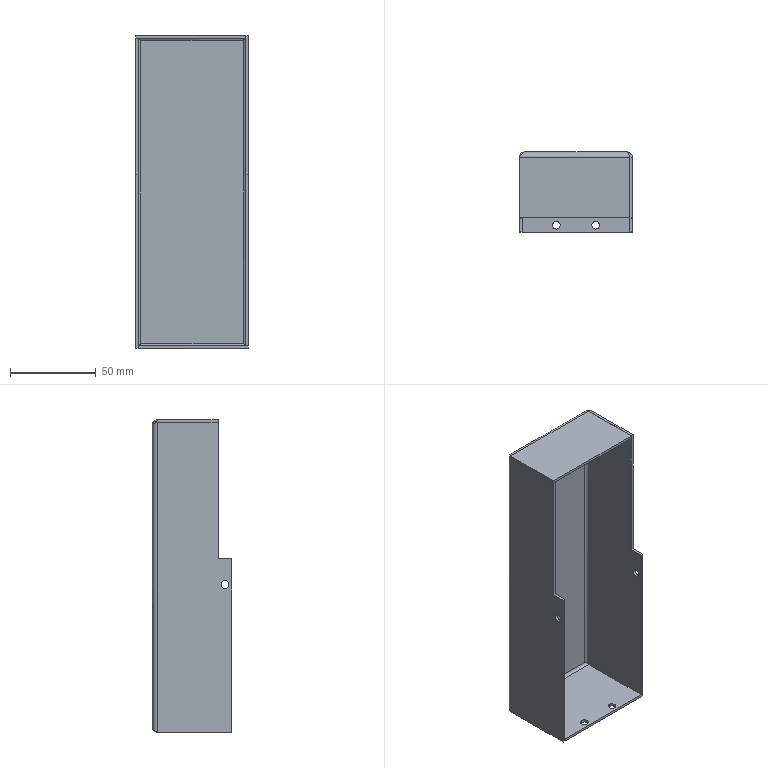Part | STEP file | 866-BDO024-95-06A | 1 solid | 50 faces | box 66 x 46.5 x 183 mm | volume 47761 mm3 | plane 26 | cylinder 16 | spline 8 | commonest cylinder face diameters 4.5 x8 3 x4 6 x4